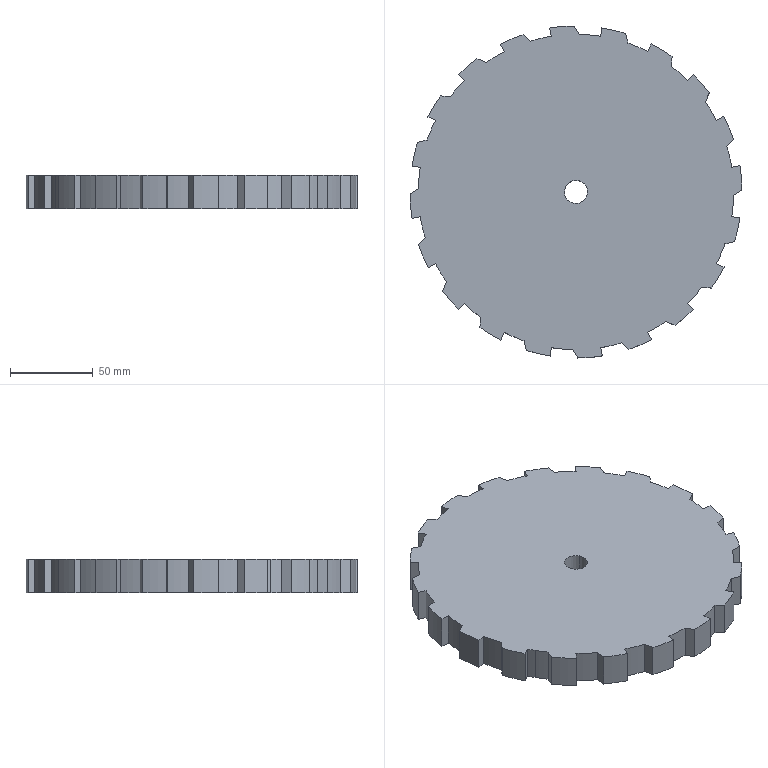Part | SolidWorks | features BaseBody 1 | 1 solid | 85 faces | box 199.988 x 199.988 x 20 mm | volume 595746 mm3 | cylinder 43 | plane 42 | commonest cylinder face diameters 190 x21 200 x20 14 x2